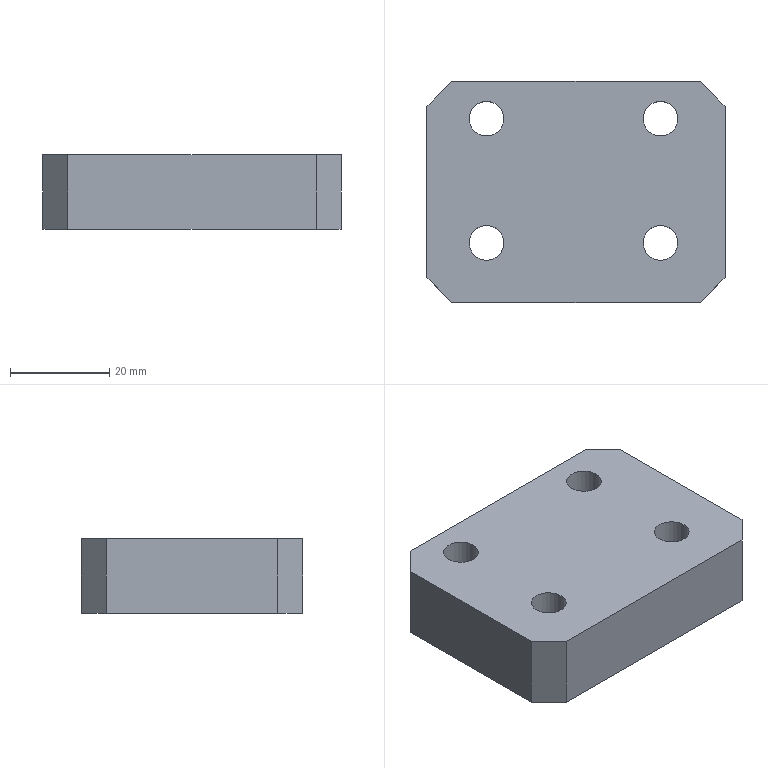Part | NX | features BREP 1 | 1 solid | 14 faces | box 60 x 44.5 x 15 mm | volume 36991 mm3 | plane 10 | cylinder 4 | commonest cylinder face diameters 7 x4
STEP:
#1=CARTESIAN_POINT('',(30.,-17.25,0.));
#2=VERTEX_POINT('',#1);
#3=CARTESIAN_POINT('',(30.,17.25,0.));
#4=VERTEX_POINT('',#3);
#5=CARTESIAN_POINT('',(30.,22.25,0.));
#6=DIRECTION('',(0.,1.,0.));
#7=VECTOR('',#6,1000.);
#8=LINE('',#5,#7);
#9=EDGE_CURVE('',#2,#4,#8,.T.);
#10=ORIENTED_EDGE('',*,*,#9,.F.);
#11=CARTESIAN_POINT('',(30.,-17.25,-15.));
#12=VERTEX_POINT('',#11);
#13=CARTESIAN_POINT('',(30.,-17.25,-15.));
#14=DIRECTION('',(0.,0.,1.));
#15=VECTOR('',#14,1000.);
#16=LINE('',#13,#15);
#17=EDGE_CURVE('',#12,#2,#16,.T.);
#18=ORIENTED_EDGE('',*,*,#17,.F.);
#19=CARTESIAN_POINT('',(30.,17.25,-15.));
#20=VERTEX_POINT('',#19);
#21=CARTESIAN_POINT('',(30.,22.25,-15.));
#22=DIRECTION('',(0.,1.,0.));
#23=VECTOR('',#22,1000.);
#24=LINE('',#21,#23);
#25=EDGE_CURVE('',#12,#20,#24,.T.);
#26=ORIENTED_EDGE('',*,*,#25,.T.);
#27=CARTESIAN_POINT('',(30.,17.25,-15.));
#28=DIRECTION('',(0.,0.,-1.));
#29=VECTOR('',#28,1000.);
#30=LINE('',#27,#29);
#31=EDGE_CURVE('',#4,#20,#30,.T.);
#32=ORIENTED_EDGE('',*,*,#31,.F.);
#33=EDGE_LOOP('',(#10,#18,#26,#32));
#34=FACE_BOUND('',#33,.T.);
#35=CARTESIAN_POINT('',(30.,22.25,-15.));
#36=DIRECTION('',(-1.,0.,0.));
#37=DIRECTION('',(0.,1.,0.));
#38=AXIS2_PLACEMENT_3D('',#35,#36,#37);
#39=PLANE('',#38);
#40=ADVANCED_FACE('',(#34),#39,.F.);
#41=CARTESIAN_POINT('',(25.,22.25,0.));
#42=VERTEX_POINT('',#41);
#43=CARTESIAN_POINT('',(-25.,22.25,0.));
#44=VERTEX_POINT('',#43);
#45=CARTESIAN_POINT('',(-30.,22.25,0.));
#46=DIRECTION('',(-1.,0.,0.));
#47=VECTOR('',#46,1000.);
#48=LINE('',#45,#47);
#49=EDGE_CURVE('',#42,#44,#48,.T.);
#50=ORIENTED_EDGE('',*,*,#49,.F.);
#51=CARTESIAN_POINT('',(25.,22.25,-15.));
#52=VERTEX_POINT('',#51);
#53=CARTESIAN_POINT('',(25.,22.25,-15.));
#54=DIRECTION('',(0.,0.,1.));
#55=VECTOR('',#54,1000.);
#56=LINE('',#53,#55);
#57=EDGE_CURVE('',#52,#42,#56,.T.);
#58=ORIENTED_EDGE('',*,*,#57,.F.);
#59=CARTESIAN_POINT('',(-25.,22.25,-15.));
#60=VERTEX_POINT('',#59);
#61=CARTESIAN_POINT('',(-30.,22.25,-15.));
#62=DIRECTION('',(-1.,0.,0.));
#63=VECTOR('',#62,1000.);
#64=LINE('',#61,#63);
#65=EDGE_CURVE('',#52,#60,#64,.T.);
#66=ORIENTED_EDGE('',*,*,#65,.T.);
#67=CARTESIAN_POINT('',(-25.,22.25,-15.));
#68=DIRECTION('',(0.,0.,-1.));
#69=VECTOR('',#68,1000.);
#70=LINE('',#67,#69);
#71=EDGE_CURVE('',#44,#60,#70,.T.);
#72=ORIENTED_EDGE('',*,*,#71,.F.);
#73=EDGE_LOOP('',(#50,#58,#66,#72));
#74=FACE_BOUND('',#73,.T.);
#75=CARTESIAN_POINT('',(-30.,22.25,-15.));
#76=DIRECTION('',(0.,-1.,0.));
#77=DIRECTION('',(0.,0.,-1.));
#78=AXIS2_PLACEMENT_3D('',#75,#76,#77);
#79=PLANE('',#78);
#80=ADVANCED_FACE('',(#74),#79,.F.);
#81=CARTESIAN_POINT('',(-30.,17.25,-15.));
#82=VERTEX_POINT('',#81);
#83=CARTESIAN_POINT('',(-30.,-17.25,-15.));
#84=VERTEX_POINT('',#83);
#85=CARTESIAN_POINT('',(-30.,22.25,-15.));
#86=DIRECTION('',(0.,-1.,0.));
#87=VECTOR('',#86,1000.);
#88=LINE('',#85,#87);
#89=EDGE_CURVE('',#82,#84,#88,.T.);
#90=ORIENTED_EDGE('',*,*,#89,.T.);
#91=CARTESIAN_POINT('',(-30.,-17.25,0.));
#92=VERTEX_POINT('',#91);
#93=CARTESIAN_POINT('',(-30.,-17.25,-15.));
#94=DIRECTION('',(0.,0.,-1.));
#95=VECTOR('',#94,1000.);
#96=LINE('',#93,#95);
#97=EDGE_CURVE('',#92,#84,#96,.T.);
#98=ORIENTED_EDGE('',*,*,#97,.F.);
#99=CARTESIAN_POINT('',(-30.,17.25,0.));
#100=VERTEX_POINT('',#99);
#101=CARTESIAN_POINT('',(-30.,22.25,0.));
#102=DIRECTION('',(0.,-1.,0.));
#103=VECTOR('',#102,1000.);
#104=LINE('',#101,#103);
#105=EDGE_CURVE('',#100,#92,#104,.T.);
#106=ORIENTED_EDGE('',*,*,#105,.F.);
#107=CARTESIAN_POINT('',(-30.,17.25,-15.));
#108=DIRECTION('',(0.,0.,1.));
#109=VECTOR('',#108,1000.);
#110=LINE('',#107,#109);
#111=EDGE_CURVE('',#82,#100,#110,.T.);
#112=ORIENTED_EDGE('',*,*,#111,.F.);
#113=EDGE_LOOP('',(#90,#98,#106,#112));
#114=FACE_BOUND('',#113,.T.);
#115=CARTESIAN_POINT('',(-30.,22.25,-15.));
#116=DIRECTION('',(1.,0.,0.));
#117=DIRECTION('',(0.,-1.,0.));
#118=AXIS2_PLACEMENT_3D('',#115,#116,#117);
#119=PLANE('',#118);
#120=ADVANCED_FACE('',(#114),#119,.F.);
#121=CARTESIAN_POINT('',(-25.,-22.25,-15.));
#122=VERTEX_POINT('',#121);
#123=CARTESIAN_POINT('',(25.,-22.25,-15.));
#124=VERTEX_POINT('',#123);
#125=CARTESIAN_POINT('',(-30.,-22.25,-15.));
#126=DIRECTION('',(1.,0.,0.));
#127=VECTOR('',#126,1000.);
#128=LINE('',#125,#127);
#129=EDGE_CURVE('',#122,#124,#128,.T.);
#130=ORIENTED_EDGE('',*,*,#129,.T.);
#131=CARTESIAN_POINT('',(25.,-22.25,0.));
#132=VERTEX_POINT('',#131);
#133=CARTESIAN_POINT('',(25.,-22.25,-15.));
#134=DIRECTION('',(0.,0.,-1.));
#135=VECTOR('',#134,1000.);
#136=LINE('',#133,#135);
#137=EDGE_CURVE('',#132,#124,#136,.T.);
#138=ORIENTED_EDGE('',*,*,#137,.F.);
#139=CARTESIAN_POINT('',(-25.,-22.25,0.));
#140=VERTEX_POINT('',#139);
#141=CARTESIAN_POINT('',(-30.,-22.25,0.));
#142=DIRECTION('',(1.,0.,0.));
#143=VECTOR('',#142,1000.);
#144=LINE('',#141,#143);
#145=EDGE_CURVE('',#140,#132,#144,.T.);
#146=ORIENTED_EDGE('',*,*,#145,.F.);
#147=CARTESIAN_POINT('',(-25.,-22.25,-15.));
#148=DIRECTION('',(0.,0.,1.));
#149=VECTOR('',#148,1000.);
#150=LINE('',#147,#149);
#151=EDGE_CURVE('',#122,#140,#150,.T.);
#152=ORIENTED_EDGE('',*,*,#151,.F.);
#153=EDGE_LOOP('',(#130,#138,#146,#152));
#154=FACE_BOUND('',#153,.T.);
#155=CARTESIAN_POINT('',(-30.,-22.25,-15.));
#156=DIRECTION('',(0.,1.,0.));
#157=DIRECTION('',(0.,0.,1.));
#158=AXIS2_PLACEMENT_3D('',#155,#156,#157);
#159=PLANE('',#158);
#160=ADVANCED_FACE('',(#154),#159,.F.);
#161=CARTESIAN_POINT('',(13.5,-10.25,-15.));
#162=VERTEX_POINT('',#161);
#163=CARTESIAN_POINT('',(17.,-10.25,-15.));
#164=DIRECTION('',(0.,0.,-1.));
#165=DIRECTION('',(-1.,0.,0.));
#166=AXIS2_PLACEMENT_3D('',#163,#164,#165);
#167=CIRCLE('',#166,3.5);
#168=EDGE_CURVE('',#162,#162,#167,.T.);
#169=ORIENTED_EDGE('',*,*,#168,.F.);
#170=EDGE_LOOP('',(#169));
#171=FACE_BOUND('',#170,.T.);
#172=CARTESIAN_POINT('',(13.5,14.75,-15.));
#173=VERTEX_POINT('',#172);
#174=CARTESIAN_POINT('',(17.,14.75,-15.));
#175=DIRECTION('',(0.,0.,-1.));
#176=DIRECTION('',(-1.,0.,0.));
#177=AXIS2_PLACEMENT_3D('',#174,#175,#176);
#178=CIRCLE('',#177,3.5);
#179=EDGE_CURVE('',#173,#173,#178,.T.);
#180=ORIENTED_EDGE('',*,*,#179,.F.);
#181=EDGE_LOOP('',(#180));
#182=FACE_BOUND('',#181,.T.);
#183=CARTESIAN_POINT('',(-21.5,14.75,-15.));
#184=VERTEX_POINT('',#183);
#185=CARTESIAN_POINT('',(-18.,14.75,-15.));
#186=DIRECTION('',(0.,0.,-1.));
#187=DIRECTION('',(-1.,0.,0.));
#188=AXIS2_PLACEMENT_3D('',#185,#186,#187);
#189=CIRCLE('',#188,3.5);
#190=EDGE_CURVE('',#184,#184,#189,.T.);
#191=ORIENTED_EDGE('',*,*,#190,.F.);
#192=EDGE_LOOP('',(#191));
#193=FACE_BOUND('',#192,.T.);
#194=CARTESIAN_POINT('',(-21.5,-10.25,-15.));
#195=VERTEX_POINT('',#194);
#196=CARTESIAN_POINT('',(-18.,-10.25,-15.));
#197=DIRECTION('',(0.,0.,-1.));
#198=DIRECTION('',(-1.,0.,0.));
#199=AXIS2_PLACEMENT_3D('',#196,#197,#198);
#200=CIRCLE('',#199,3.5);
#201=EDGE_CURVE('',#195,#195,#200,.T.);
#202=ORIENTED_EDGE('',*,*,#201,.F.);
#203=EDGE_LOOP('',(#202));
#204=FACE_BOUND('',#203,.T.);
#205=ORIENTED_EDGE('',*,*,#65,.F.);
#206=CARTESIAN_POINT('',(23.625,23.625,-15.));
#207=DIRECTION('',(-0.7071,0.7071,0.));
#208=VECTOR('',#207,1000.);
#209=LINE('',#206,#208);
#210=EDGE_CURVE('',#20,#52,#209,.T.);
#211=ORIENTED_EDGE('',*,*,#210,.F.);
#212=ORIENTED_EDGE('',*,*,#25,.F.);
#213=CARTESIAN_POINT('',(23.625,-23.625,-15.));
#214=DIRECTION('',(0.7071,0.7071,0.));
#215=VECTOR('',#214,1000.);
#216=LINE('',#213,#215);
#217=EDGE_CURVE('',#124,#12,#216,.T.);
#218=ORIENTED_EDGE('',*,*,#217,.F.);
#219=ORIENTED_EDGE('',*,*,#129,.F.);
#220=CARTESIAN_POINT('',(-23.625,-23.625,-15.));
#221=DIRECTION('',(0.7071,-0.7071,0.));
#222=VECTOR('',#221,1000.);
#223=LINE('',#220,#222);
#224=EDGE_CURVE('',#84,#122,#223,.T.);
#225=ORIENTED_EDGE('',*,*,#224,.F.);
#226=ORIENTED_EDGE('',*,*,#89,.F.);
#227=CARTESIAN_POINT('',(-23.625,23.625,-15.));
#228=DIRECTION('',(-0.7071,-0.7071,0.));
#229=VECTOR('',#228,1000.);
#230=LINE('',#227,#229);
#231=EDGE_CURVE('',#60,#82,#230,.T.);
#232=ORIENTED_EDGE('',*,*,#231,.F.);
#233=EDGE_LOOP('',(#205,#211,#212,#218,#219,#225,#226,#232));
#234=FACE_BOUND('',#233,.T.);
#235=CARTESIAN_POINT('',(0.,0.,-15.));
#236=DIRECTION('',(0.,0.,-1.));
#237=DIRECTION('',(-1.,0.,0.));
#238=AXIS2_PLACEMENT_3D('',#235,#236,#237);
#239=PLANE('',#238);
#240=ADVANCED_FACE('',(#171,#182,#193,#204,#234),#239,.T.);
#241=CARTESIAN_POINT('',(13.5,-10.25,0.));
#242=VERTEX_POINT('',#241);
#243=CARTESIAN_POINT('',(17.,-10.25,0.));
#244=DIRECTION('',(0.,0.,-1.));
#245=DIRECTION('',(-1.,0.,0.));
#246=AXIS2_PLACEMENT_3D('',#243,#244,#245);
#247=CIRCLE('',#246,3.5);
#248=EDGE_CURVE('',#242,#242,#247,.T.);
#249=ORIENTED_EDGE('',*,*,#248,.T.);
#250=EDGE_LOOP('',(#249));
#251=FACE_BOUND('',#250,.T.);
#252=CARTESIAN_POINT('',(13.5,14.75,0.));
#253=VERTEX_POINT('',#252);
#254=CARTESIAN_POINT('',(17.,14.75,0.));
#255=DIRECTION('',(0.,0.,-1.));
#256=DIRECTION('',(-1.,0.,0.));
#257=AXIS2_PLACEMENT_3D('',#254,#255,#256);
#258=CIRCLE('',#257,3.5);
#259=EDGE_CURVE('',#253,#253,#258,.T.);
#260=ORIENTED_EDGE('',*,*,#259,.T.);
#261=EDGE_LOOP('',(#260));
#262=FACE_BOUND('',#261,.T.);
#263=CARTESIAN_POINT('',(-21.5,14.75,0.));
#264=VERTEX_POINT('',#263);
#265=CARTESIAN_POINT('',(-18.,14.75,0.));
#266=DIRECTION('',(0.,0.,-1.));
#267=DIRECTION('',(-1.,0.,0.));
#268=AXIS2_PLACEMENT_3D('',#265,#266,#267);
#269=CIRCLE('',#268,3.5);
#270=EDGE_CURVE('',#264,#264,#269,.T.);
#271=ORIENTED_EDGE('',*,*,#270,.T.);
#272=EDGE_LOOP('',(#271));
#273=FACE_BOUND('',#272,.T.);
#274=CARTESIAN_POINT('',(-21.5,-10.25,0.));
#275=VERTEX_POINT('',#274);
#276=CARTESIAN_POINT('',(-18.,-10.25,0.));
#277=DIRECTION('',(0.,0.,-1.));
#278=DIRECTION('',(-1.,0.,0.));
#279=AXIS2_PLACEMENT_3D('',#276,#277,#278);
#280=CIRCLE('',#279,3.5);
#281=EDGE_CURVE('',#275,#275,#280,.T.);
#282=ORIENTED_EDGE('',*,*,#281,.T.);
#283=EDGE_LOOP('',(#282));
#284=FACE_BOUND('',#283,.T.);
#285=ORIENTED_EDGE('',*,*,#105,.T.);
#286=CARTESIAN_POINT('',(-25.,-22.25,0.));
#287=DIRECTION('',(-0.7071,0.7071,0.));
#288=VECTOR('',#287,1000.);
#289=LINE('',#286,#288);
#290=EDGE_CURVE('',#140,#92,#289,.T.);
#291=ORIENTED_EDGE('',*,*,#290,.F.);
#292=ORIENTED_EDGE('',*,*,#145,.T.);
#293=CARTESIAN_POINT('',(30.,-17.25,0.));
#294=DIRECTION('',(-0.7071,-0.7071,0.));
#295=VECTOR('',#294,1000.);
#296=LINE('',#293,#295);
#297=EDGE_CURVE('',#2,#132,#296,.T.);
#298=ORIENTED_EDGE('',*,*,#297,.F.);
#299=ORIENTED_EDGE('',*,*,#9,.T.);
#300=CARTESIAN_POINT('',(25.,22.25,0.));
#301=DIRECTION('',(0.7071,-0.7071,0.));
#302=VECTOR('',#301,1000.);
#303=LINE('',#300,#302);
#304=EDGE_CURVE('',#42,#4,#303,.T.);
#305=ORIENTED_EDGE('',*,*,#304,.F.);
#306=ORIENTED_EDGE('',*,*,#49,.T.);
#307=CARTESIAN_POINT('',(-30.,17.25,0.));
#308=DIRECTION('',(0.7071,0.7071,0.));
#309=VECTOR('',#308,1000.);
#310=LINE('',#307,#309);
#311=EDGE_CURVE('',#100,#44,#310,.T.);
#312=ORIENTED_EDGE('',*,*,#311,.F.);
#313=EDGE_LOOP('',(#285,#291,#292,#298,#299,#305,#306,#312));
#314=FACE_BOUND('',#313,.T.);
#315=CARTESIAN_POINT('',(0.,0.,0.));
#316=DIRECTION('',(0.,0.,-1.));
#317=DIRECTION('',(-1.,0.,0.));
#318=AXIS2_PLACEMENT_3D('',#315,#316,#317);
#319=PLANE('',#318);
#320=ADVANCED_FACE('',(#251,#262,#273,#284,#314),#319,.F.);
#321=ORIENTED_EDGE('',*,*,#201,.T.);
#322=EDGE_LOOP('',(#321));
#323=FACE_BOUND('',#322,.T.);
#324=ORIENTED_EDGE('',*,*,#281,.F.);
#325=EDGE_LOOP('',(#324));
#326=FACE_BOUND('',#325,.T.);
#327=CARTESIAN_POINT('',(-18.,-10.25,0.));
#328=DIRECTION('',(0.,0.,1.));
#329=DIRECTION('',(1.,0.,0.));
#330=AXIS2_PLACEMENT_3D('',#327,#328,#329);
#331=CYLINDRICAL_SURFACE('',#330,3.5);
#332=ADVANCED_FACE('',(#323,#326),#331,.F.);
#333=ORIENTED_EDGE('',*,*,#190,.T.);
#334=EDGE_LOOP('',(#333));
#335=FACE_BOUND('',#334,.T.);
#336=ORIENTED_EDGE('',*,*,#270,.F.);
#337=EDGE_LOOP('',(#336));
#338=FACE_BOUND('',#337,.T.);
#339=CARTESIAN_POINT('',(-18.,14.75,0.));
#340=DIRECTION('',(0.,0.,1.));
#341=DIRECTION('',(1.,0.,0.));
#342=AXIS2_PLACEMENT_3D('',#339,#340,#341);
#343=CYLINDRICAL_SURFACE('',#342,3.5);
#344=ADVANCED_FACE('',(#335,#338),#343,.F.);
#345=ORIENTED_EDGE('',*,*,#179,.T.);
#346=EDGE_LOOP('',(#345));
#347=FACE_BOUND('',#346,.T.);
#348=ORIENTED_EDGE('',*,*,#259,.F.);
#349=EDGE_LOOP('',(#348));
#350=FACE_BOUND('',#349,.T.);
#351=CARTESIAN_POINT('',(17.,14.75,0.));
#352=DIRECTION('',(0.,0.,1.));
#353=DIRECTION('',(1.,0.,0.));
#354=AXIS2_PLACEMENT_3D('',#351,#352,#353);
#355=CYLINDRICAL_SURFACE('',#354,3.5);
#356=ADVANCED_FACE('',(#347,#350),#355,.F.);
#357=ORIENTED_EDGE('',*,*,#168,.T.);
#358=EDGE_LOOP('',(#357));
#359=FACE_BOUND('',#358,.T.);
#360=ORIENTED_EDGE('',*,*,#248,.F.);
#361=EDGE_LOOP('',(#360));
#362=FACE_BOUND('',#361,.T.);
#363=CARTESIAN_POINT('',(17.,-10.25,0.));
#364=DIRECTION('',(0.,0.,1.));
#365=DIRECTION('',(1.,0.,0.));
#366=AXIS2_PLACEMENT_3D('',#363,#364,#365);
#367=CYLINDRICAL_SURFACE('',#366,3.5);
#368=ADVANCED_FACE('',(#359,#362),#367,.F.);
#369=ORIENTED_EDGE('',*,*,#231,.T.);
#370=ORIENTED_EDGE('',*,*,#111,.T.);
#371=ORIENTED_EDGE('',*,*,#311,.T.);
#372=ORIENTED_EDGE('',*,*,#71,.T.);
#373=EDGE_LOOP('',(#369,#370,#371,#372));
#374=FACE_BOUND('',#373,.T.);
#375=CARTESIAN_POINT('',(-30.,17.25,-15.));
#376=DIRECTION('',(0.7071,-0.7071,0.));
#377=DIRECTION('',(0.,0.,-1.));
#378=AXIS2_PLACEMENT_3D('',#375,#376,#377);
#379=PLANE('',#378);
#380=ADVANCED_FACE('',(#374),#379,.F.);
#381=ORIENTED_EDGE('',*,*,#210,.T.);
#382=ORIENTED_EDGE('',*,*,#57,.T.);
#383=ORIENTED_EDGE('',*,*,#304,.T.);
#384=ORIENTED_EDGE('',*,*,#31,.T.);
#385=EDGE_LOOP('',(#381,#382,#383,#384));
#386=FACE_BOUND('',#385,.T.);
#387=CARTESIAN_POINT('',(25.,22.25,-15.));
#388=DIRECTION('',(-0.7071,-0.7071,0.));
#389=DIRECTION('',(0.,0.,-1.));
#390=AXIS2_PLACEMENT_3D('',#387,#388,#389);
#391=PLANE('',#390);
#392=ADVANCED_FACE('',(#386),#391,.F.);
#393=ORIENTED_EDGE('',*,*,#224,.T.);
#394=ORIENTED_EDGE('',*,*,#151,.T.);
#395=ORIENTED_EDGE('',*,*,#290,.T.);
#396=ORIENTED_EDGE('',*,*,#97,.T.);
#397=EDGE_LOOP('',(#393,#394,#395,#396));
#398=FACE_BOUND('',#397,.T.);
#399=CARTESIAN_POINT('',(-25.,-22.25,-15.));
#400=DIRECTION('',(0.7071,0.7071,0.));
#401=DIRECTION('',(0.,0.,-1.));
#402=AXIS2_PLACEMENT_3D('',#399,#400,#401);
#403=PLANE('',#402);
#404=ADVANCED_FACE('',(#398),#403,.F.);
#405=ORIENTED_EDGE('',*,*,#217,.T.);
#406=ORIENTED_EDGE('',*,*,#17,.T.);
#407=ORIENTED_EDGE('',*,*,#297,.T.);
#408=ORIENTED_EDGE('',*,*,#137,.T.);
#409=EDGE_LOOP('',(#405,#406,#407,#408));
#410=FACE_BOUND('',#409,.T.);
#411=CARTESIAN_POINT('',(30.,-17.25,-15.));
#412=DIRECTION('',(-0.7071,0.7071,0.));
#413=DIRECTION('',(0.,0.,-1.));
#414=AXIS2_PLACEMENT_3D('',#411,#412,#413);
#415=PLANE('',#414);
#416=ADVANCED_FACE('',(#410),#415,.F.);
#417=CLOSED_SHELL('',(#40,#80,#120,#160,#240,#320,#332,#344,#356,#368,#380,#392,#404,#416));
#418=MANIFOLD_SOLID_BREP('',#417);
#419=(LENGTH_UNIT()NAMED_UNIT(*)SI_UNIT(.MILLI.,.METRE.));
#420=UNCERTAINTY_MEASURE_WITH_UNIT(LENGTH_MEASURE(0.00001),#419,'','');
#421=(NAMED_UNIT(*)PLANE_ANGLE_UNIT()SI_UNIT($,.RADIAN.));
#422=(NAMED_UNIT(*)SI_UNIT($,.STERADIAN.)SOLID_ANGLE_UNIT());
#423=(GEOMETRIC_REPRESENTATION_CONTEXT(3)GLOBAL_UNCERTAINTY_ASSIGNED_CONTEXT((#420))GLOBAL_UNIT_ASSIGNED_CONTEXT((#419,#421,#422))REPRESENTATION_CONTEXT('',''));
#424=ADVANCED_BREP_SHAPE_REPRESENTATION('',(#418),#423);